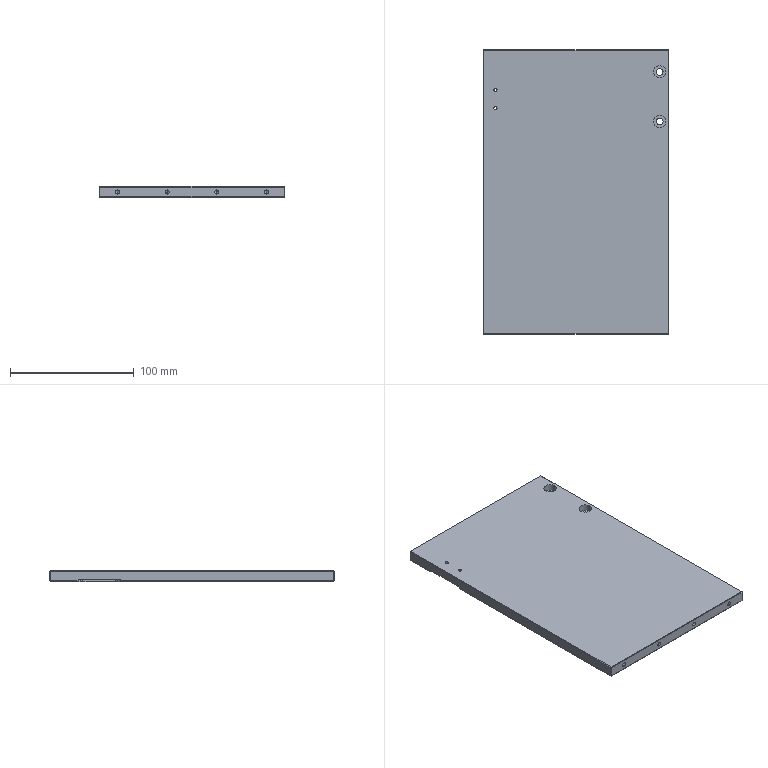Part | STEP file | BPSP-11-002Unloading Support Plate1_Default | 1 solid | 81 faces | box 150 x 230 x 9 mm | volume 307149 mm3 | plane 35 | cylinder 30 | cone 16 | commonest cylinder face diameters 3.3 x16 2.5 x4 5.5 x4 10 x4 4 x2